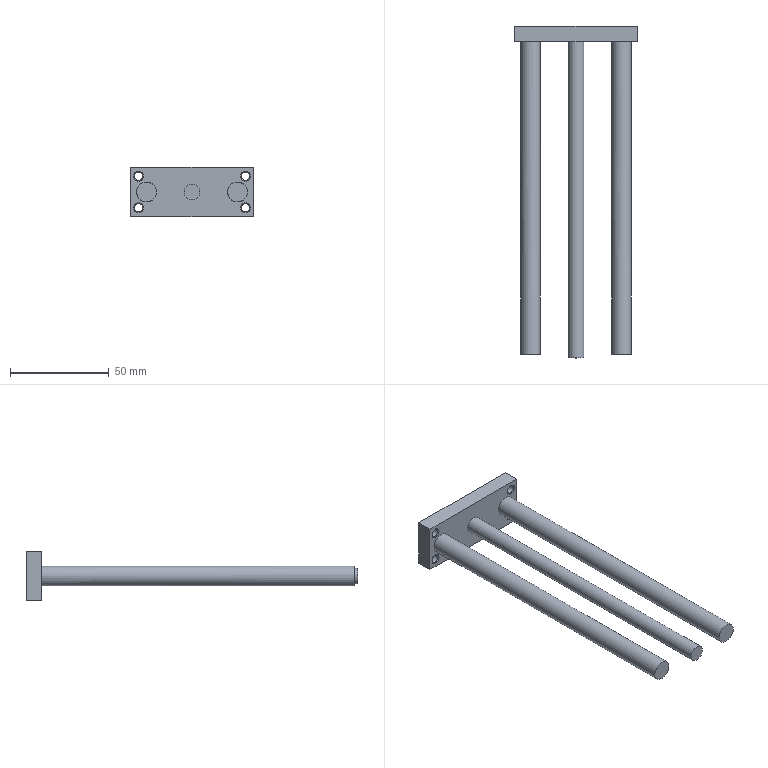Part | STEP file | Tube necking machine_id22_x_t | 1 solid | 24 faces | box 62 x 167.8 x 25 mm | volume 44767 mm3 | plane 9 | cone 8 | cylinder 7 | commonest cylinder face diameters 4.2 x4 10 x2 8 x1